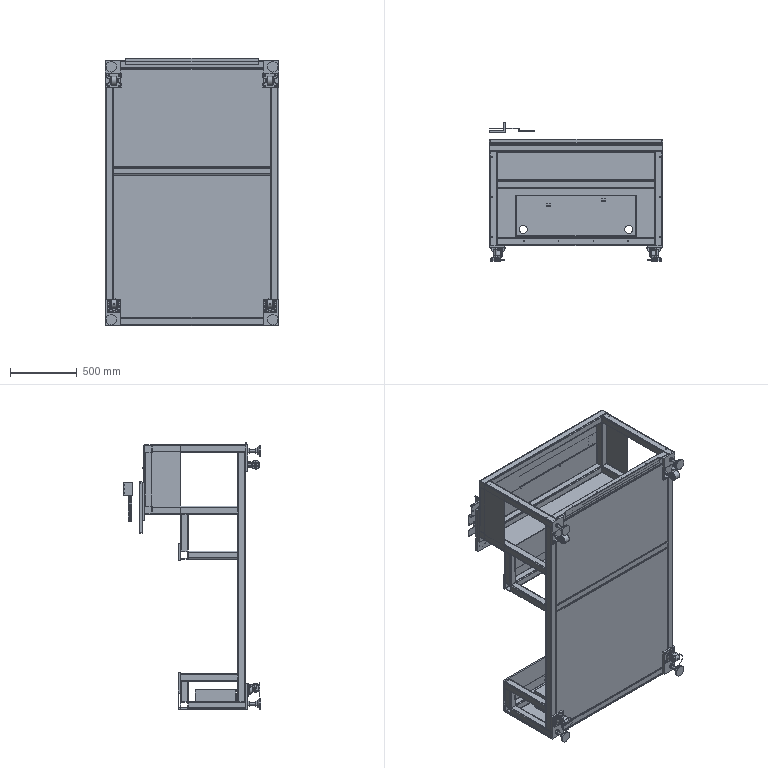Part | NX | features BREP 49 | 62 solids | 2556 faces | box 1303 x 1034 x 2009 mm | volume 48407621 mm3 | cylinder 1159 | plane 923 | cone 350 | torus 92 | spline 32 | commonest cylinder face diameters 5 x244 8 x126 16 x116 3.3 x102 4 x67 8.5 x56